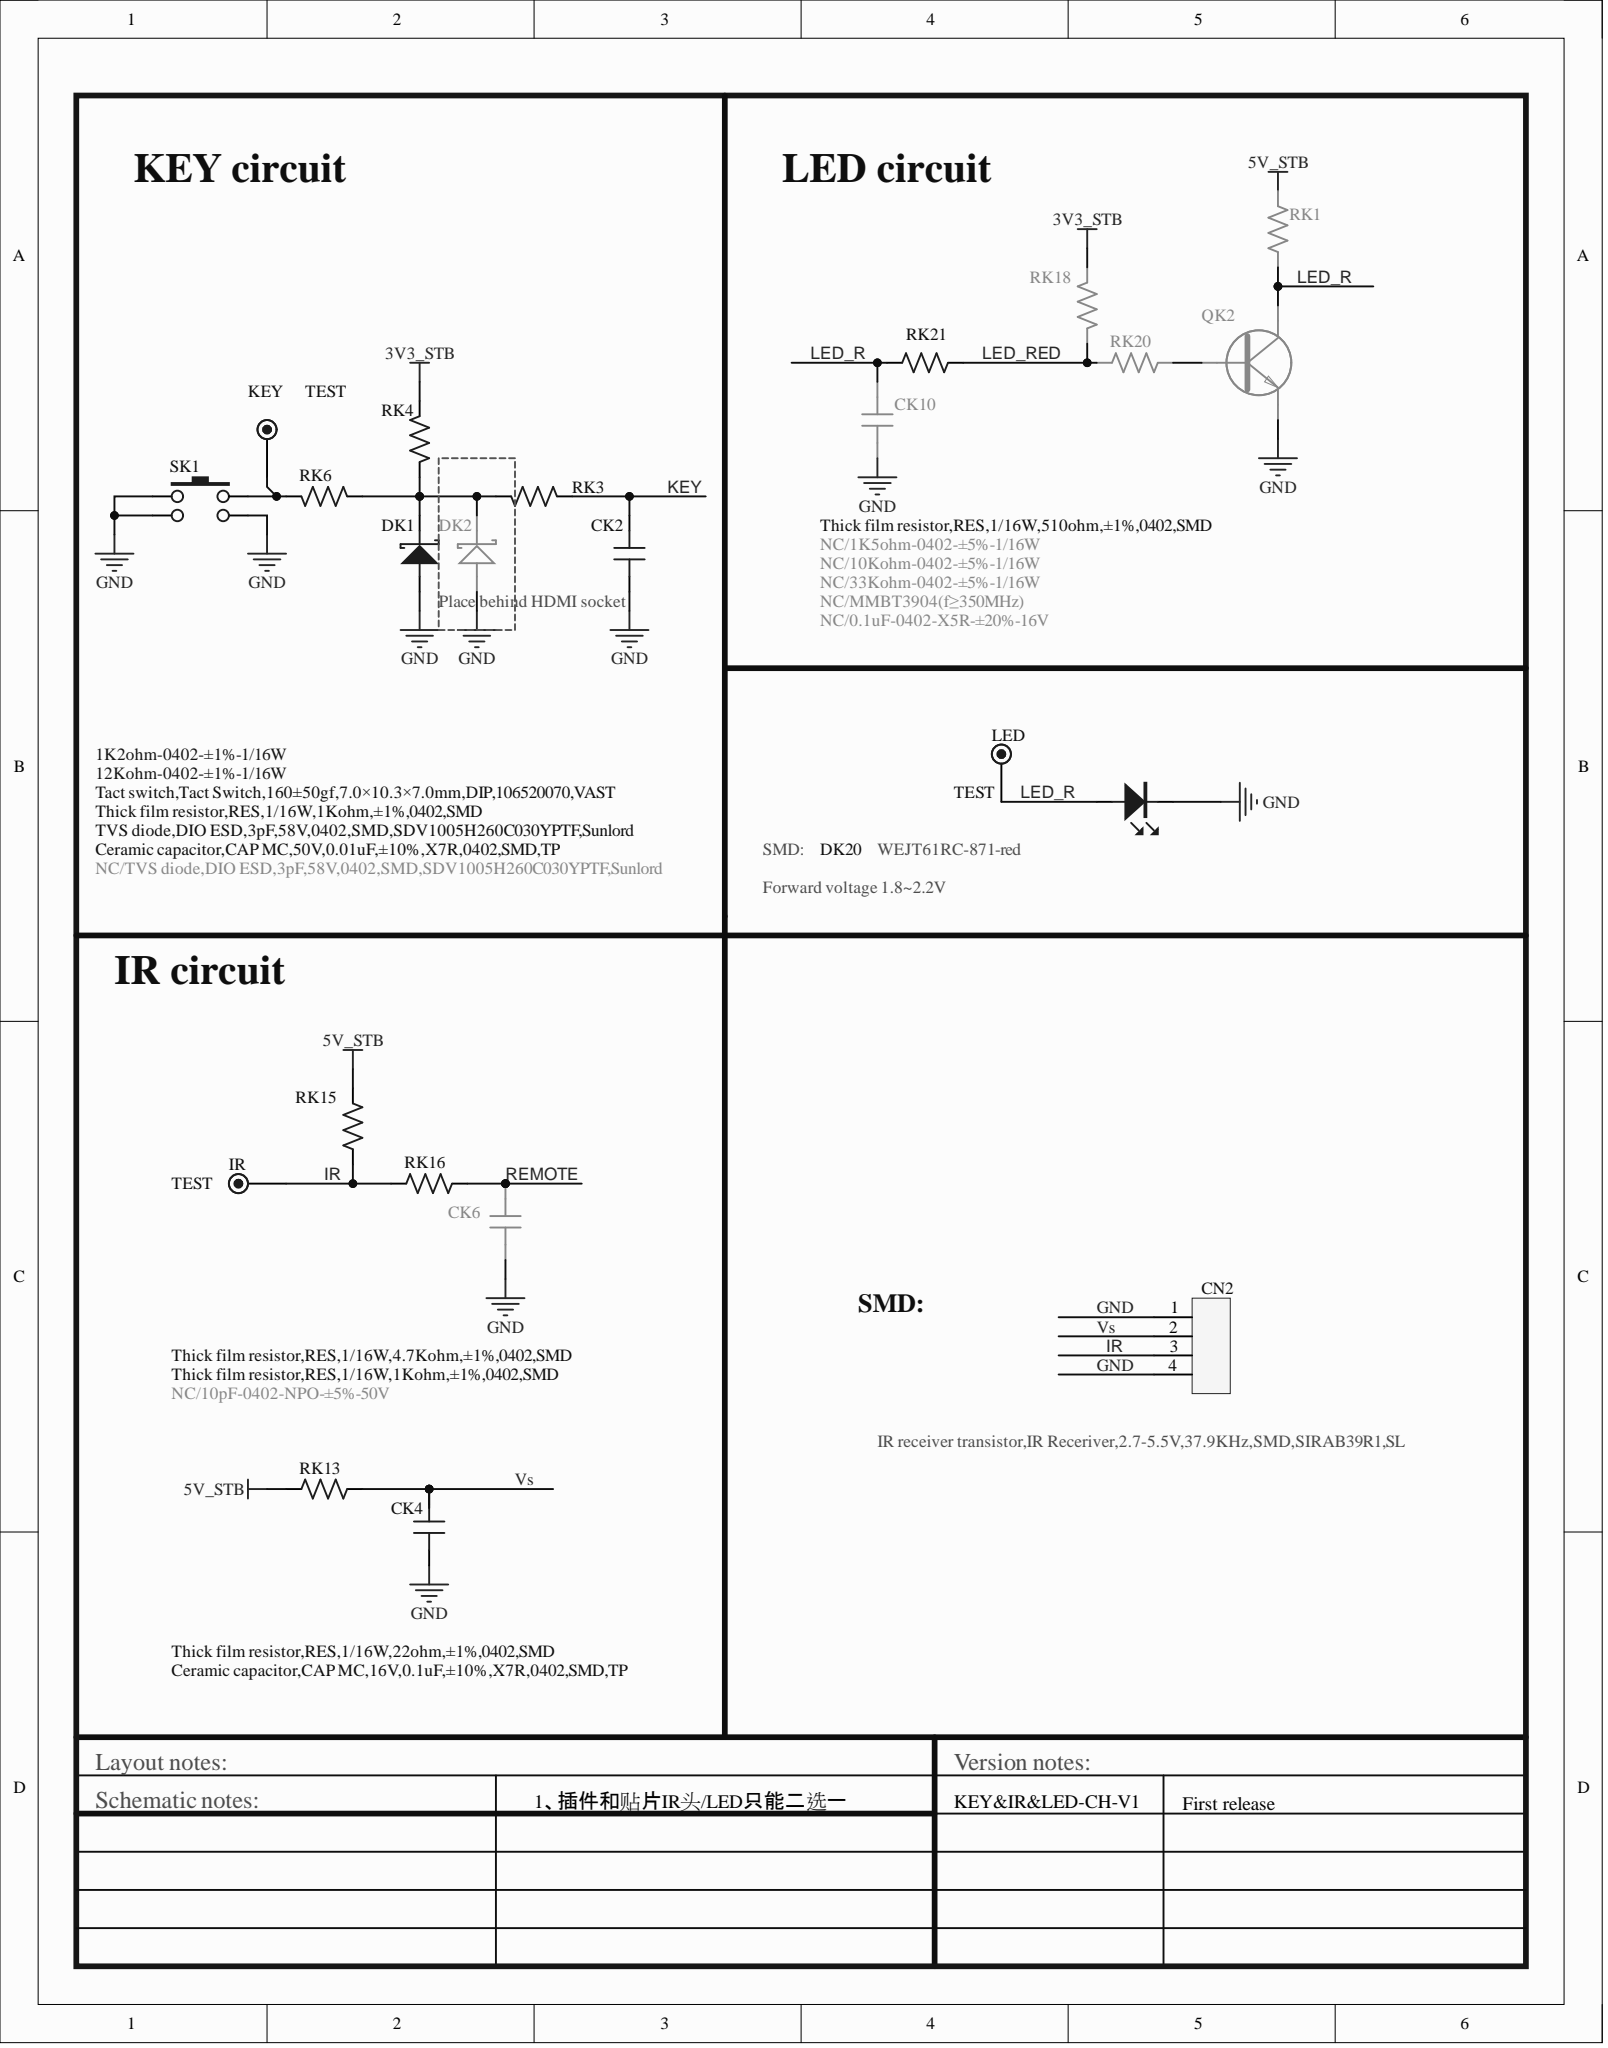Circuit board | Altium Designer | 719 parts | 352 nets | one sheet of the schematic
Parts on this sheet (reference | value | footprint):
CK2 | Ceramic capacitor,CAP MC,50V,0.01uF,±10%,X7R,0402,SMD,TP | C0402
CK4 | Ceramic capacitor,CAP MC,16V,0.1uF,±10%,X7R,0402,SMD,TP | C0402
CK6 | NC/10pF-0402-NPO-±5%-50V | C0402
CK10 | NC/0.1uF-0402-X5R-±20%-16V | C0402
CN2 | IR receiver transistor,IR Receriver,2.7-5.5V,37.9KHz,SMD,SIRAB39R1,SL | REMOTE-HS-1
DK1 | TVS diode,DIO ESD,3pF,58V,0402,SMD,SDV1005H260C030YPTF,Sunlord | DIODE-S0402
DK2 | NC/TVS diode,DIO ESD,3pF,58V,0402,SMD,SDV1005H260C030YPTF,Sunlord | DIODE-S0402
DK20 | WEJT61RC-871-red | DIODE-S0603
IR | TEST | TP
KEY | TEST | TP
LED | TEST | TP
QK2 | NC/MMBT3904(f=350MHz) | SOT-23
RK1 | NC/1K5ohm-0402-±5%-1/16W | R0402
RK3 | Thick film resistor,RES,1/16W,1Kohm,±1%,0402,SMD | R0402
RK4 | 12Kohm-0402-±1%-1/16W | R0402
RK6 | 1K2ohm-0402-±1%-1/16W | R0402
RK13 | Thick film resistor,RES,1/16W,22ohm,±1%,0402,SMD | R0402
RK15 | Thick film resistor,RES,1/16W,4.7Kohm,±1%,0402,SMD | R0402
RK16 | Thick film resistor,RES,1/16W,1Kohm,±1%,0402,SMD | R0402
RK18 | NC/33Kohm-0402-±5%-1/16W | R0402
RK20 | NC/10Kohm-0402-±5%-1/16W | R0402
RK21 | Thick film resistor,RES,1/16W,510ohm,±1%,0402,SMD | R0402
SK1 | Tact switch,Tact Switch,160±50gf,7.0×10.3×7.0mm,DIP,106520070,VAST | KEY-HD-6
Nets of these parts (net: part-pin ...):
Vs: CK4-1 CN2-2 RK13-2
REMOTE: CK6-2 RK16-1
NetQK2_B: QK2-B RK20-1
NetKEY_1: KEY-1 RK6-2 SK1-2
NetDK1_K: DK1-K DK2-K RK3-2 RK4-1 RK6-1
LED_RED: RK18-1 RK20-2 RK21-1
LED_R: CK10-2 DK20-A LED-1 QK2-C RK1-1 RK21-2
KEY: CK2-1 RK3-1
IR: CN2-3 IR-1 RK15-2 RK16-2
GND: CK2-2 CK4-2 CK6-1 CK10-1 CN2-1 CN2-4 DK1-A DK2-A DK20-K QK2-E SK1-1 SK1-3 SK1-4
5V_STB: RK1-2 RK13-1 RK15-1
3V3_STB: RK4-2 RK18-2